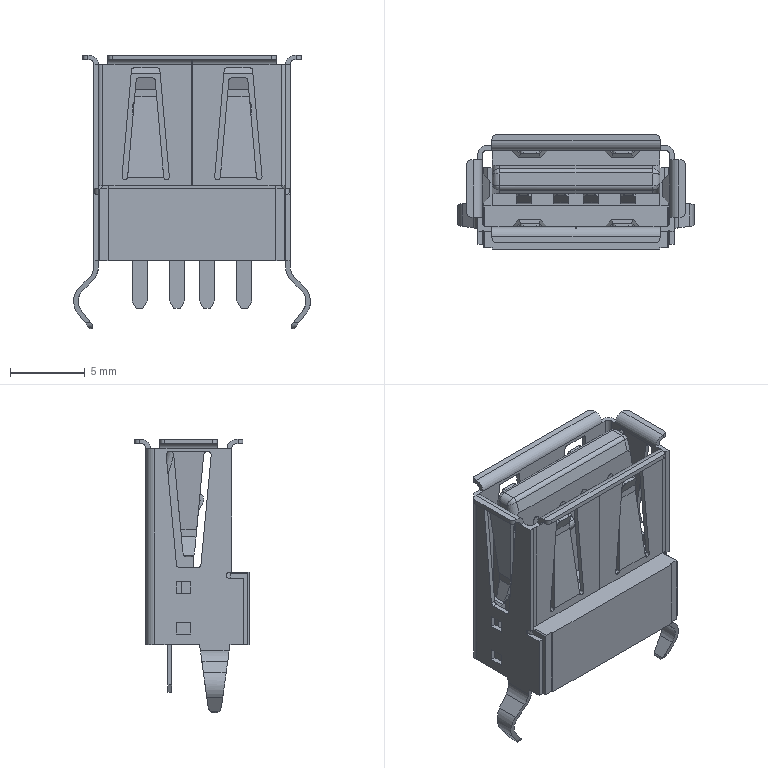Part | SolidWorks | features BaseBody 1 | 1 solid | 470 faces | box 15.807 x 7.64 x 18.249 mm | volume 686.202 mm3 | plane 329 | cylinder 137 | spline 4 | commonest cylinder face diameters 0.4 x30 1 x26 0.313 x16 0.6 x14 0.5 x12 0.312 x8